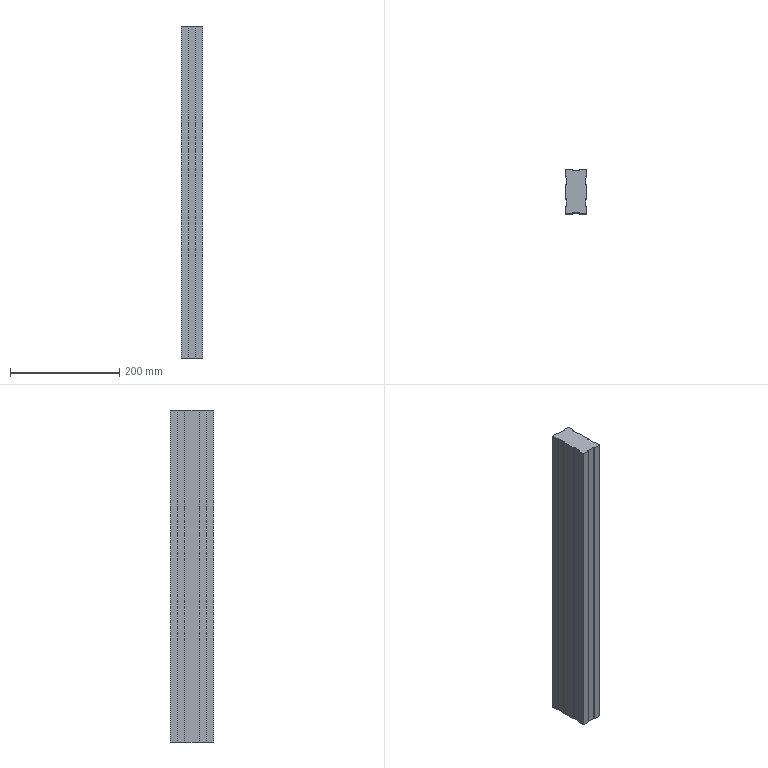Part | STEP file | xingcai40x80x800 | 1 solid | 30 faces | box 40 x 80 x 609 mm | volume 1846488 mm3 | plane 30